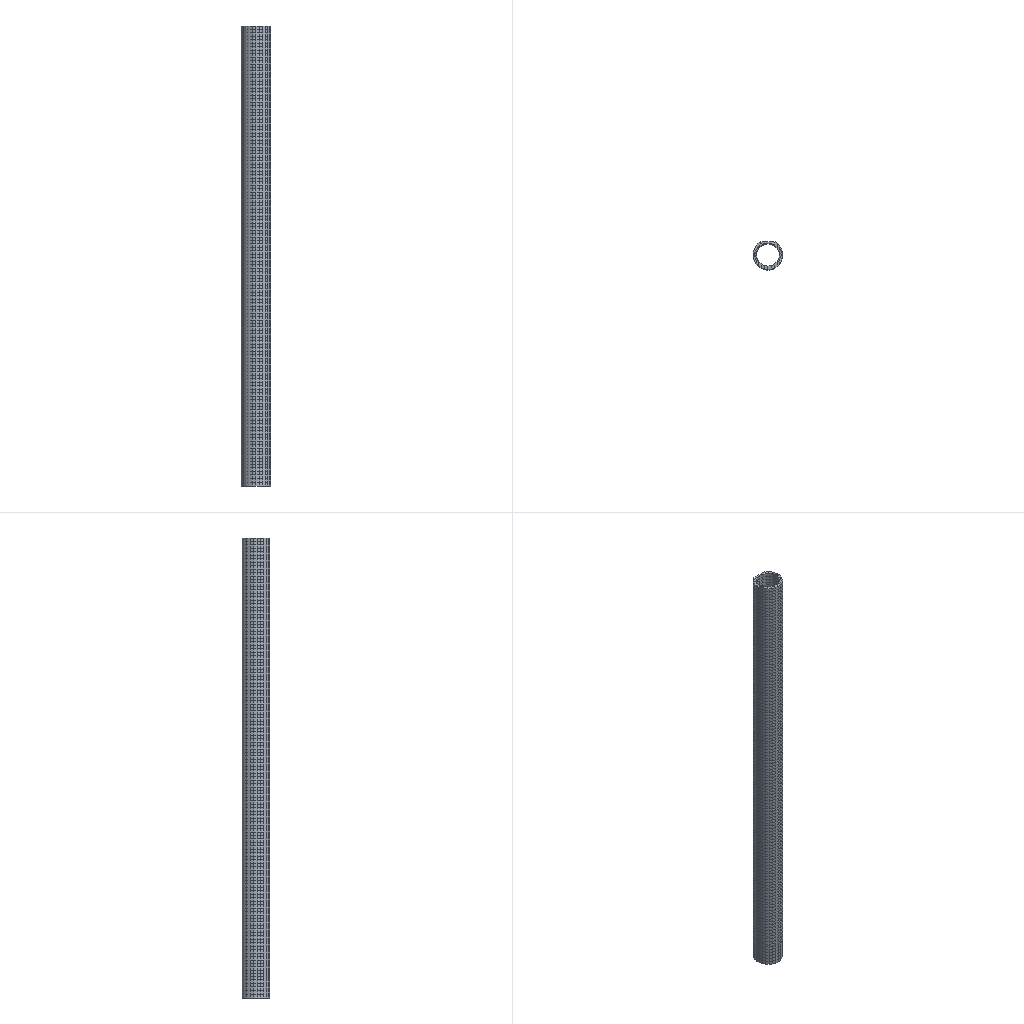Simulation study | abaqus
Set-up summary:
category,name,step,type,value,unit,region
solver,abaqus,,Abaqus/CAE 2024
units,mm-N-s-tonne (MPa),,inferred,E=210000 density=
analysis,Step-4,,static,time_period=10
mesh,nodes,,,9381
mesh,elements,,,6118
element_type,C3D8R,,,6118
material,Material-1,,E,210000
material,Material-1,,nu,0.3
material,Material-1,,yield,380
material,Material-1,,cte,1.3e-05
material,Material-1,,behaviors,plastic; expansion
section,Material-1,,solid section,,,Set-1
load,Load-2,Step-4,pressure,30,,Surf-6
load,Load-4,Step-4,concentrated force,"1000 [dir=(0, 1, 0)]",,Set-13
bc,BC-1,initial,fixed,"[dofs=rx,ry,rz,x,y,z n=6]",,Set-5
bc,BC-2,Step-4,displacement,-0.5 [dofs=rx],,_PickedSet34
bc,BC-2,Step-4,fixed,"[dofs=ry,rz n=2]",,_PickedSet34
constraint,coupling,,,1
Abaqus input file, long lists of numbers shortened:
*Heading
** Job name: deck Model name: Model-1-4
** Generated by: Abaqus/CAE 2024
*Preprint, echo=NO, model=NO, history=NO, contact=NO
**
** PARTS
**
*Part, name=Part-10
*Node
      1,           0.,          56.,         120.
      2,           0.,          50.,         120.
** (9378 more lines like these left out)
*Element, type=C3D8R
   1,    2,   33,   51,    1,  299,  991, 2107,   52
   2,    7,   51,   33,   34,  547, 2107,  991,  992
** (6116 more lines like these left out)
*Nset, nset=Set-1, generate
    1,  9380,     1
*Elset, elset=Set-1, generate
    1,  6118,     1
** Section: Section-1
*Solid Section, elset=Set-1, material=Material-1
,
*End Part
**
**
** ASSEMBLY
**
*Assembly, name=Assembly
**
*Instance, name=Part-10-1, part=Part-10
*End Instance
**
*Node
      1,           0., -3.91886993e-15,        2000.
*Nset, nset=Set-5, instance=Part-10-1
   22,   23,   24,   25,   26,   30,   31,   32,  908,  909,  910,  911,  912,  913,  914,  915
  916,  917,  918,  919,  920,  921,  922,  923,  924,  925,  926,  927,  928,  954,  955,  956
** (3 more lines like these left out)
*Elset, elset=Set-5, instance=Part-10-1
 5926, 5927, 5928, 5929, 5930, 5931, 5932, 5933, 5934, 5935, 5936, 5937, 5938, 5939, 5940, 5941
 5942, 5943, 5944, 5945, 5946, 5947, 5948, 5949, 5950, 6098, 6099, 6100, 6101, 6102, 6103, 6104
** (1 more lines like these left out)
*Nset, nset=Set-13
 1,
*Nset, nset=m_Set-12
 1,
*Nset, nset=s_Set-8, instance=Part-10-1
    8,    9,   10,   11,   12,   13,   14,   16,  672,  673,  674,  675,  676,  677,  678,  679
  680,  681,  682,  683,  684,  685,  686,  687,  688,  689,  690,  836,  837,  838,  839,  840
** (3 more lines like these left out)
*Elset, elset=s_Set-8, instance=Part-10-1
 2605, 2606, 2607, 2608, 2609, 2610, 2611, 2612, 2613, 2614, 2615, 2616, 2617, 2618, 2619, 2620
 2621, 2622, 2623, 2624, 2625, 5726, 5727, 5728, 5729, 5730, 5731, 5732, 5733, 5734, 5735, 5736
** (1 more lines like these left out)
*Nset, nset=_PickedSet34, internal
 1,
*Elset, elset=_Surf-2_S3, internal, instance=Part-10-1
    1,    3,   22,   24,   43,   45,   64,   66,   85,   87,  106,  108,  127,  129,  148,  150
  169,  171,  190,  192,  211,  213,  232,  234,  253,  255,  274,  276,  295,  297,  316,  318
** (33 more lines like these left out)
*Elset, elset=_Surf-2_S4, internal, instance=Part-10-1
    6,    9,   10,   11,   20,   27,   30,   31,   32,   41,   48,   51,   52,   53,   62,   69
   72,   73,   74,   83,   90,   93,   94,   95,  104,  111,  114,  115,  116,  125,  132,  135
** (40 more lines like these left out)
*Elset, elset=_Surf-2_S6, internal, instance=Part-10-1
   17,   19,   38,   40,   59,   61,   80,   82,  101,  103,  122,  124,  143,  145,  164,  166
  185,  187,  206,  208,  227,  229,  248,  250,  269,  271,  290,  292,  311,  313,  332,  334
** (47 more lines like these left out)
*Elset, elset=_Surf-2_S5, internal, instance=Part-10-1
    2,   23,   44,   65,   86,  107,  128,  149,  170,  191,  212,  233,  254,  275,  296,  317
  338,  359,  380,  401,  422,  443,  464,  485,  506,  527,  548,  569,  590,  611,  632,  653
** (40 more lines like these left out)
*Surface, type=ELEMENT, name=Surf-2
_Surf-2_S3, S3
_Surf-2_S4, S4
_Surf-2_S6, S6
_Surf-2_S5, S5
*Elset, elset=_Surf-5_S4, internal, instance=Part-10-1
    8,   29,   50,   71,   92,  113,  134,  155,  176,  197,  218,  239,  260,  281,  302,  323
  344,  365,  386,  407,  428,  449,  470,  491,  512,  533,  554,  575,  596,  617,  638,  659
** (17 more lines like these left out)
*Elset, elset=_Surf-5_S6, internal, instance=Part-10-1
    9,   10,   11,   14,   30,   31,   32,   35,   51,   52,   53,   56,   72,   73,   74,   77
   93,   94,   95,   98,  114,  115,  116,  119,  135,  136,  137,  140,  156,  157,  158,  161
** (39 more lines like these left out)
*Elset, elset=_Surf-5_S3, internal, instance=Part-10-1
    4,    5,   15,   25,   26,   36,   46,   47,   57,   67,   68,   78,   88,   89,   99,  109
  110,  120,  130,  131,  141,  151,  152,  162,  172,  173,  183,  193,  194,  204,  214,  215
** (47 more lines like these left out)
*Elset, elset=_Surf-5_S5, internal, instance=Part-10-1
    3,   12,   13,   16,   24,   33,   34,   37,   45,   54,   55,   58,   66,   75,   76,   79
   87,   96,   97,  100,  108,  117,  118,  121,  129,  138,  139,  142,  150,  159,  160,  163
** (77 more lines like these left out)
*Surface, type=ELEMENT, name=Surf-5
_Surf-5_S4, S4
_Surf-5_S6, S6
_Surf-5_S3, S3
_Surf-5_S5, S5
*Elset, elset=_Surf-6_S4, internal, instance=Part-10-1
    8,   29,   50,   71,   92,  113,  134,  155,  176,  197,  218,  239,  260,  281,  302,  323
  344,  365,  386,  407,  428,  449,  470,  491,  512,  533,  554,  575,  596,  617,  638,  659
** (28 more lines like these left out)
*Elset, elset=_Surf-6_S6, internal, instance=Part-10-1
    9,   10,   11,   14,   30,   31,   32,   35,   51,   52,   53,   56,   72,   73,   74,   77
   93,   94,   95,   98,  114,  115,  116,  119,  135,  136,  137,  140,  156,  157,  158,  161
** (41 more lines like these left out)
*Elset, elset=_Surf-6_S5, internal, instance=Part-10-1
    1,    3,   12,   13,   16,   22,   24,   33,   34,   37,   43,   45,   54,   55,   58,   64
   66,   75,   76,   79,   85,   87,   96,   97,  100,  106,  108,  117,  118,  121,  127,  129
** (102 more lines like these left out)
*Elset, elset=_Surf-6_S3, internal, instance=Part-10-1
    2,    4,    5,   15,   23,   25,   26,   36,   44,   46,   47,   57,   65,   67,   68,   78
   86,   88,   89,   99,  107,  109,  110,  120,  128,  130,  131,  141,  149,  151,  152,  162
** (56 more lines like these left out)
*Surface, type=ELEMENT, name=Surf-6
_Surf-6_S4, S4
_Surf-6_S6, S6
_Surf-6_S5, S5
_Surf-6_S3, S3
*Elset, elset=_m_Surf-3_S2, internal, instance=Part-10-1
 2605, 2606, 2607, 2608, 2609, 2610, 2611, 2612, 2613, 2614, 2615, 2616, 2617, 2618, 2619, 2620
 2621, 2622, 2623, 2624, 2625, 5726, 5727, 5728, 5729, 5730, 5731, 5732, 5733, 5734, 5735, 5736
** (1 more lines like these left out)
*Surface, type=ELEMENT, name=m_Surf-3
_m_Surf-3_S2, S2
*Elset, elset=_s_Surf-4_S2, internal, instance=Part-10-1
 2605, 2606, 2607, 2608, 2609, 2610, 2611, 2612, 2613, 2614, 2615, 2616, 2617, 2618, 2619, 2620
 2621, 2622, 2623, 2624, 2625, 5726, 5727, 5728, 5729, 5730, 5731, 5732, 5733, 5734, 5735, 5736
** (1 more lines like these left out)
*Surface, type=ELEMENT, name=s_Surf-4
_s_Surf-4_S2, S2
** Constraint: Constraint-3
*Coupling, constraint name=Constraint-3, ref node=m_Set-12, surface=s_Surf-4
*Kinematic
*End Assembly
**
** MATERIALS
**
*Material, name=Material-1
*Elastic
210000., 0.3
*Expansion
 1.3e-05,
*Plastic
380.,  0.
600., 0.2
**
** BOUNDARY CONDITIONS
**
** Name: BC-1 Type: Displacement/Rotation
*Boundary
Set-5, 1, 1
Set-5, 2, 2
Set-5, 3, 3
Set-5, 4, 4
Set-5, 5, 5
Set-5, 6, 6
** ----------------------------------------------------------------
**
** STEP: Step-4
**
*Step, name=Step-4, nlgeom=NO, inc=1000
*Static
1., 10., 0.0001, 1.
**
** BOUNDARY CONDITIONS
**
** Name: BC-2 Type: Displacement/Rotation
*Boundary
_PickedSet34, 4, 4, -0.5
_PickedSet34, 5, 5
_PickedSet34, 6, 6
**
** LOADS
**
** Name: Load-2   Type: Pressure
*Dsload
Surf-6, P, 30.
** Name: Load-4   Type: Concentrated force
*Cload
Set-13, 2, 1000.
**
** OUTPUT REQUESTS
**
*Restart, write, frequency=0
**
** FIELD OUTPUT: F-Output-2
**
*Output, field
*Node Output
CF, RF, RM, RT, TF, U, UR, UT
V, VF, VR, VT
*Element Output, directions=YES
ALPHA, ALPHAN, BF, CENTMAG, CENTRIFMAG, CORIOMAG, CS11, CTSHR, E, EE, EEQUT, ER, ESF1, GRAV, HP, IE
LE, LODE, MISES, MISESMAX, MISESONLY, NE, NFORC, NFORCSO, P, PE, PEEQ, PEEQMAX, PEEQT, PEMAG, PEQC, PRESSONLY
PS, ROTAMAG, S, SALPHA, SE, SEE, SEP, SEPE, SEQUT, SF, SPE, SQEQ, SSAVG, TE, TEEQ, TEVOL
THE, TRIAX, TRNOR, TRSHR, TSHR, VE, VEEQ, VS, YIELDPOT
**
** HISTORY OUTPUT: H-Output-2
**
*Output, history
*Element Output
IRA1, IRA2, IRA3, IRAR1, IRAR2, IRAR3, IRF1, IRF2, IRF3, IRM1, IRM2, IRM3
*End Step
Results summary:
result,odb.job_status,,,JOB_STATUS_COMPLETED_SUCCESSFULLY,"consistent, unstated (Abaqus has no unit system)"
result,steps[0].procedure,Step-4,,*STATIC,"consistent, unstated (Abaqus has no unit system)"
result,steps[0].time_period,Step-4,,10,"consistent, unstated (Abaqus has no unit system)"
result,steps[0].n_frames,Step-4,,11,"consistent, unstated (Abaqus has no unit system)"
result,steps[0].last_frame.id,Step-4,,10,"consistent, unstated (Abaqus has no unit system)"
result,steps[0].last_frame.value,Step-4,,10,"consistent, unstated (Abaqus has no unit system)"
result,steps[0].last_frame.description,Step-4,,Increment     10: Step Time =    10.00,"consistent, unstated (Abaqus has no unit system)"
result,steps[0].completed,Step-4,,True,"consistent, unstated (Abaqus has no unit system)"
result,steps[0].max_U_magnitude,Step-4,,558.326,"consistent, unstated (Abaqus has no unit system)"
result,steps[0].max_S_mises,Step-4,,403.668,"consistent, unstated (Abaqus has no unit system)"
result,steps[0].RF_sum[1],Step-4,,0.008606,"consistent, unstated (Abaqus has no unit system)"
result,steps[0].RF_sum[2],Step-4,,-1000.02,"consistent, unstated (Abaqus has no unit system)"
result,steps[0].RF_sum[3],Step-4,,0.06396,"consistent, unstated (Abaqus has no unit system)"